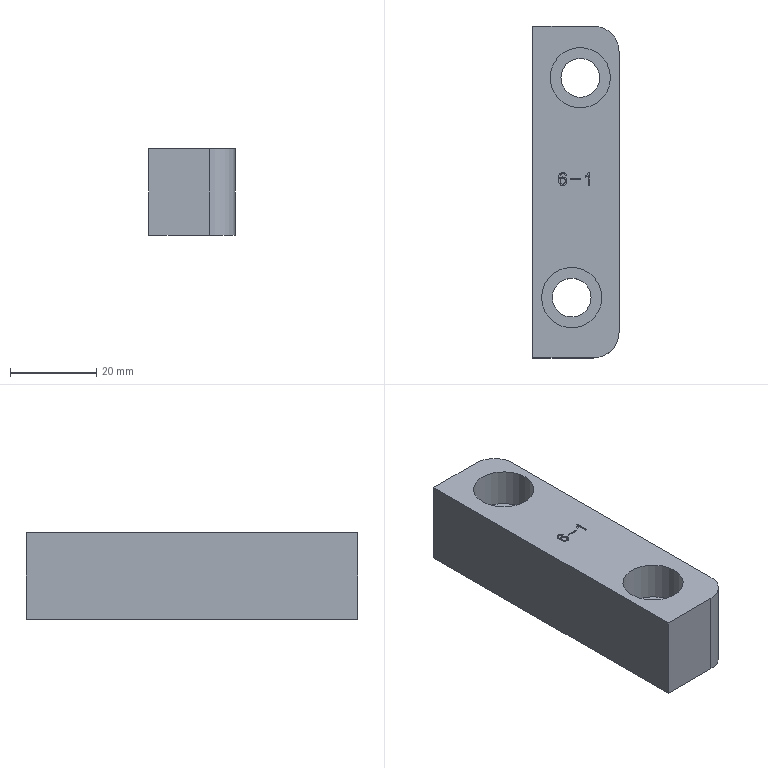Part | STEP file | solid 13 | 1 solid | 34 faces | box 20 x 76.984 x 20 mm | volume 26313 mm3 | plane 22 | cylinder 6 | other 6 | commonest cylinder face diameters 9 x2 12 x2 14 x2